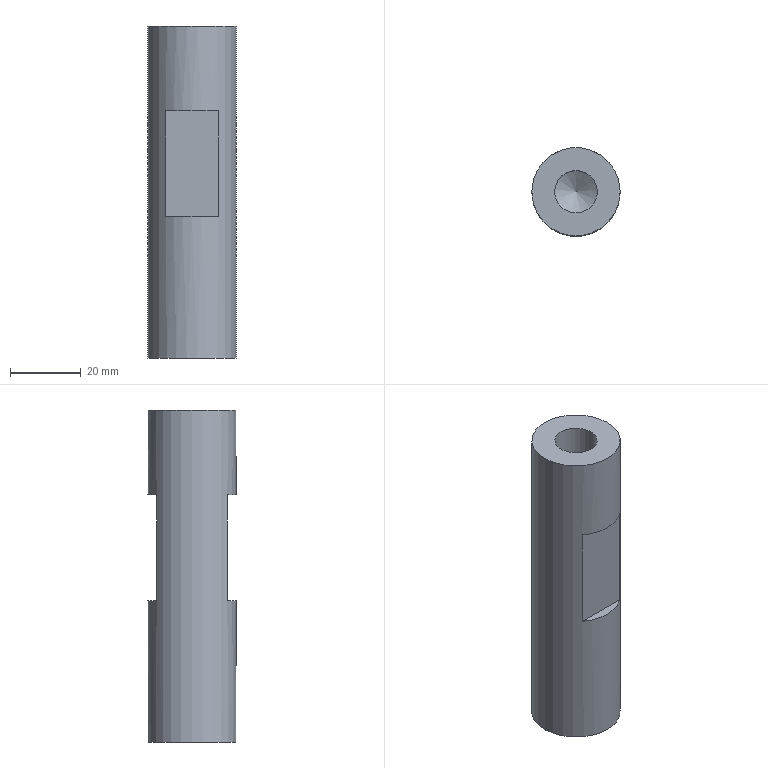Part | NX | features solid 2 | 1 solid | 13 faces | box 25 x 25 x 94 mm | volume 38683 mm3 | plane 8 | cylinder 3 | cone 2 | commonest cylinder face diameters 12 x2 25 x1
STEP:
#1=CARTESIAN_POINT('',(657.5,75.,-75.));
#2=VERTEX_POINT('',#1);
#3=CARTESIAN_POINT('',(670.,75.,-75.));
#4=DIRECTION('',(0.,0.,-1.));
#5=DIRECTION('',(-1.,0.,0.));
#6=AXIS2_PLACEMENT_3D('',#3,#4,#5);
#7=CIRCLE('',#6,12.5);
#8=EDGE_CURVE('',#2,#2,#7,.F.);
#9=ORIENTED_EDGE('',*,*,#8,.F.);
#10=EDGE_LOOP('',(#9));
#11=FACE_BOUND('',#10,.T.);
#12=CARTESIAN_POINT('',(682.5,75.,-169.));
#13=VERTEX_POINT('',#12);
#14=CARTESIAN_POINT('',(670.,75.,-169.));
#15=DIRECTION('',(0.,0.,1.));
#16=DIRECTION('',(1.,0.,0.));
#17=AXIS2_PLACEMENT_3D('',#14,#15,#16);
#18=CIRCLE('',#17,12.5);
#19=EDGE_CURVE('',#13,#13,#18,.T.);
#20=ORIENTED_EDGE('',*,*,#19,.T.);
#21=EDGE_LOOP('',(#20));
#22=FACE_BOUND('',#21,.T.);
#23=CARTESIAN_POINT('',(677.5,85.,-99.));
#24=VERTEX_POINT('',#23);
#25=CARTESIAN_POINT('',(677.5,85.,-129.));
#26=VERTEX_POINT('',#25);
#27=CARTESIAN_POINT('',(677.5,85.,-99.));
#28=DIRECTION('',(0.,0.,1.));
#29=VECTOR('',#28,1000.);
#30=LINE('',#27,#29);
#31=EDGE_CURVE('',#24,#26,#30,.F.);
#32=ORIENTED_EDGE('',*,*,#31,.F.);
#33=CARTESIAN_POINT('',(662.5,85.,-99.));
#34=VERTEX_POINT('',#33);
#35=CARTESIAN_POINT('',(670.,75.,-99.));
#36=DIRECTION('',(0.,0.,-1.));
#37=DIRECTION('',(-1.,0.,0.));
#38=AXIS2_PLACEMENT_3D('',#35,#36,#37);
#39=CIRCLE('',#38,12.5);
#40=EDGE_CURVE('',#34,#24,#39,.T.);
#41=ORIENTED_EDGE('',*,*,#40,.F.);
#42=CARTESIAN_POINT('',(662.5,85.,-129.));
#43=VERTEX_POINT('',#42);
#44=CARTESIAN_POINT('',(662.5,85.,-129.));
#45=DIRECTION('',(0.,0.,1.));
#46=VECTOR('',#45,1000.);
#47=LINE('',#44,#46);
#48=EDGE_CURVE('',#43,#34,#47,.T.);
#49=ORIENTED_EDGE('',*,*,#48,.F.);
#50=CARTESIAN_POINT('',(670.,75.,-129.));
#51=DIRECTION('',(0.,0.,-1.));
#52=DIRECTION('',(-1.,0.,0.));
#53=AXIS2_PLACEMENT_3D('',#50,#51,#52);
#54=CIRCLE('',#53,12.5);
#55=EDGE_CURVE('',#26,#43,#54,.F.);
#56=ORIENTED_EDGE('',*,*,#55,.F.);
#57=EDGE_LOOP('',(#32,#41,#49,#56));
#58=FACE_BOUND('',#57,.T.);
#59=CARTESIAN_POINT('',(662.5,65.,-99.));
#60=VERTEX_POINT('',#59);
#61=CARTESIAN_POINT('',(677.5,65.,-99.));
#62=VERTEX_POINT('',#61);
#63=CARTESIAN_POINT('',(670.,75.,-99.));
#64=DIRECTION('',(0.,0.,-1.));
#65=DIRECTION('',(-1.,0.,0.));
#66=AXIS2_PLACEMENT_3D('',#63,#64,#65);
#67=CIRCLE('',#66,12.5);
#68=EDGE_CURVE('',#60,#62,#67,.F.);
#69=ORIENTED_EDGE('',*,*,#68,.T.);
#70=CARTESIAN_POINT('',(677.5,65.,-129.));
#71=VERTEX_POINT('',#70);
#72=CARTESIAN_POINT('',(677.5,65.,-99.));
#73=DIRECTION('',(0.,0.,1.));
#74=VECTOR('',#73,1000.);
#75=LINE('',#72,#74);
#76=EDGE_CURVE('',#62,#71,#75,.F.);
#77=ORIENTED_EDGE('',*,*,#76,.T.);
#78=CARTESIAN_POINT('',(662.5,65.,-129.));
#79=VERTEX_POINT('',#78);
#80=CARTESIAN_POINT('',(670.,75.,-129.));
#81=DIRECTION('',(0.,0.,-1.));
#82=DIRECTION('',(-1.,0.,0.));
#83=AXIS2_PLACEMENT_3D('',#80,#81,#82);
#84=CIRCLE('',#83,12.5);
#85=EDGE_CURVE('',#71,#79,#84,.T.);
#86=ORIENTED_EDGE('',*,*,#85,.T.);
#87=CARTESIAN_POINT('',(662.5,65.,-129.));
#88=DIRECTION('',(0.,0.,1.));
#89=VECTOR('',#88,1000.);
#90=LINE('',#87,#89);
#91=EDGE_CURVE('',#79,#60,#90,.T.);
#92=ORIENTED_EDGE('',*,*,#91,.T.);
#93=EDGE_LOOP('',(#69,#77,#86,#92));
#94=FACE_BOUND('',#93,.T.);
#95=CARTESIAN_POINT('',(670.,75.,-169.));
#96=DIRECTION('',(0.,0.,1.));
#97=DIRECTION('',(0.,1.,0.));
#98=AXIS2_PLACEMENT_3D('',#95,#96,#97);
#99=CYLINDRICAL_SURFACE('',#98,12.5);
#100=ADVANCED_FACE('',(#11,#22,#58,#94),#99,.T.);
#101=CARTESIAN_POINT('',(670.,81.,-169.));
#102=VERTEX_POINT('',#101);
#103=CARTESIAN_POINT('',(670.,75.,-169.));
#104=DIRECTION('',(0.,0.,1.));
#105=DIRECTION('',(0.,1.,0.));
#106=AXIS2_PLACEMENT_3D('',#103,#104,#105);
#107=CIRCLE('',#106,6.);
#108=EDGE_CURVE('',#102,#102,#107,.T.);
#109=ORIENTED_EDGE('',*,*,#108,.T.);
#110=EDGE_LOOP('',(#109));
#111=FACE_BOUND('',#110,.T.);
#112=ORIENTED_EDGE('',*,*,#19,.F.);
#113=EDGE_LOOP('',(#112));
#114=FACE_BOUND('',#113,.T.);
#115=CARTESIAN_POINT('',(670.,75.,-169.));
#116=DIRECTION('',(0.,0.,1.));
#117=DIRECTION('',(0.,1.,0.));
#118=AXIS2_PLACEMENT_3D('',#115,#116,#117);
#119=PLANE('',#118);
#120=ADVANCED_FACE('',(#111,#114),#119,.F.);
#121=CARTESIAN_POINT('',(670.,69.,-75.));
#122=VERTEX_POINT('',#121);
#123=CARTESIAN_POINT('',(670.,75.,-75.));
#124=DIRECTION('',(0.,0.,-1.));
#125=DIRECTION('',(0.,-1.,0.));
#126=AXIS2_PLACEMENT_3D('',#123,#124,#125);
#127=CIRCLE('',#126,6.);
#128=EDGE_CURVE('',#122,#122,#127,.T.);
#129=ORIENTED_EDGE('',*,*,#128,.T.);
#130=EDGE_LOOP('',(#129));
#131=FACE_BOUND('',#130,.T.);
#132=ORIENTED_EDGE('',*,*,#8,.T.);
#133=EDGE_LOOP('',(#132));
#134=FACE_BOUND('',#133,.T.);
#135=CARTESIAN_POINT('',(520.,-10.,-75.));
#136=DIRECTION('',(0.,0.,-1.));
#137=DIRECTION('',(-1.,0.,0.));
#138=AXIS2_PLACEMENT_3D('',#135,#136,#137);
#139=PLANE('',#138);
#140=ADVANCED_FACE('',(#131,#134),#139,.F.);
#141=CARTESIAN_POINT('',(670.,69.,-95.));
#142=VERTEX_POINT('',#141);
#143=CARTESIAN_POINT('',(670.,75.,-95.));
#144=DIRECTION('',(0.,0.,-1.));
#145=DIRECTION('',(0.,-1.,0.));
#146=AXIS2_PLACEMENT_3D('',#143,#144,#145);
#147=CIRCLE('',#146,6.);
#148=EDGE_CURVE('',#142,#142,#147,.T.);
#149=ORIENTED_EDGE('',*,*,#148,.F.);
#150=EDGE_LOOP('',(#149));
#151=FACE_BOUND('',#150,.T.);
#152=CARTESIAN_POINT('',(670.,75.,-98.605));
#153=VERTEX_POINT('',#152);
#154=VERTEX_LOOP('',#153);
#155=FACE_BOUND('',#154,.T.);
#156=CARTESIAN_POINT('',(670.,75.,-95.));
#157=DIRECTION('',(0.,0.,1.));
#158=DIRECTION('',(0.,1.,0.));
#159=AXIS2_PLACEMENT_3D('',#156,#157,#158);
#160=CONICAL_SURFACE('',#159,6.,1.03);
#161=ADVANCED_FACE('',(#151,#155),#160,.F.);
#162=ORIENTED_EDGE('',*,*,#148,.T.);
#163=EDGE_LOOP('',(#162));
#164=FACE_BOUND('',#163,.T.);
#165=ORIENTED_EDGE('',*,*,#128,.F.);
#166=EDGE_LOOP('',(#165));
#167=FACE_BOUND('',#166,.T.);
#168=CARTESIAN_POINT('',(670.,75.,-65.));
#169=DIRECTION('',(0.,0.,-1.));
#170=DIRECTION('',(0.,-1.,0.));
#171=AXIS2_PLACEMENT_3D('',#168,#169,#170);
#172=CYLINDRICAL_SURFACE('',#171,6.);
#173=ADVANCED_FACE('',(#164,#167),#172,.F.);
#174=CARTESIAN_POINT('',(670.,81.,-139.));
#175=VERTEX_POINT('',#174);
#176=CARTESIAN_POINT('',(670.,75.,-139.));
#177=DIRECTION('',(0.,0.,1.));
#178=DIRECTION('',(0.,1.,0.));
#179=AXIS2_PLACEMENT_3D('',#176,#177,#178);
#180=CIRCLE('',#179,6.);
#181=EDGE_CURVE('',#175,#175,#180,.T.);
#182=ORIENTED_EDGE('',*,*,#181,.F.);
#183=EDGE_LOOP('',(#182));
#184=FACE_BOUND('',#183,.T.);
#185=CARTESIAN_POINT('',(670.,75.,-135.395));
#186=VERTEX_POINT('',#185);
#187=VERTEX_LOOP('',#186);
#188=FACE_BOUND('',#187,.T.);
#189=CARTESIAN_POINT('',(670.,75.,-139.));
#190=DIRECTION('',(0.,0.,-1.));
#191=DIRECTION('',(0.,-1.,0.));
#192=AXIS2_PLACEMENT_3D('',#189,#190,#191);
#193=CONICAL_SURFACE('',#192,6.,1.03);
#194=ADVANCED_FACE('',(#184,#188),#193,.F.);
#195=ORIENTED_EDGE('',*,*,#181,.T.);
#196=EDGE_LOOP('',(#195));
#197=FACE_BOUND('',#196,.T.);
#198=ORIENTED_EDGE('',*,*,#108,.F.);
#199=EDGE_LOOP('',(#198));
#200=FACE_BOUND('',#199,.T.);
#201=CARTESIAN_POINT('',(670.,75.,-169.));
#202=DIRECTION('',(0.,0.,1.));
#203=DIRECTION('',(0.,1.,0.));
#204=AXIS2_PLACEMENT_3D('',#201,#202,#203);
#205=CYLINDRICAL_SURFACE('',#204,6.);
#206=ADVANCED_FACE('',(#197,#200),#205,.F.);
#207=ORIENTED_EDGE('',*,*,#55,.T.);
#208=CARTESIAN_POINT('',(655.,85.,-129.));
#209=DIRECTION('',(1.,0.,0.));
#210=VECTOR('',#209,1000.);
#211=LINE('',#208,#210);
#212=EDGE_CURVE('',#43,#26,#211,.T.);
#213=ORIENTED_EDGE('',*,*,#212,.T.);
#214=EDGE_LOOP('',(#207,#213));
#215=FACE_BOUND('',#214,.T.);
#216=CARTESIAN_POINT('',(655.,75.,-129.));
#217=DIRECTION('',(0.,0.,-1.));
#218=DIRECTION('',(1.,0.,0.));
#219=AXIS2_PLACEMENT_3D('',#216,#217,#218);
#220=PLANE('',#219);
#221=ADVANCED_FACE('',(#215),#220,.F.);
#222=ORIENTED_EDGE('',*,*,#40,.T.);
#223=CARTESIAN_POINT('',(655.,85.,-99.));
#224=DIRECTION('',(-1.,0.,0.));
#225=VECTOR('',#224,1000.);
#226=LINE('',#223,#225);
#227=EDGE_CURVE('',#34,#24,#226,.F.);
#228=ORIENTED_EDGE('',*,*,#227,.F.);
#229=EDGE_LOOP('',(#222,#228));
#230=FACE_BOUND('',#229,.T.);
#231=CARTESIAN_POINT('',(655.,75.,-99.));
#232=DIRECTION('',(0.,0.,-1.));
#233=DIRECTION('',(1.,0.,0.));
#234=AXIS2_PLACEMENT_3D('',#231,#232,#233);
#235=PLANE('',#234);
#236=ADVANCED_FACE('',(#230),#235,.T.);
#237=ORIENTED_EDGE('',*,*,#31,.T.);
#238=ORIENTED_EDGE('',*,*,#212,.F.);
#239=ORIENTED_EDGE('',*,*,#48,.T.);
#240=ORIENTED_EDGE('',*,*,#227,.T.);
#241=EDGE_LOOP('',(#237,#238,#239,#240));
#242=FACE_BOUND('',#241,.T.);
#243=CARTESIAN_POINT('',(655.,85.,-129.));
#244=DIRECTION('',(0.,-1.,0.));
#245=DIRECTION('',(0.,0.,1.));
#246=AXIS2_PLACEMENT_3D('',#243,#244,#245);
#247=PLANE('',#246);
#248=ADVANCED_FACE('',(#242),#247,.F.);
#249=CARTESIAN_POINT('',(655.,65.,-129.));
#250=DIRECTION('',(-1.,0.,0.));
#251=VECTOR('',#250,1000.);
#252=LINE('',#249,#251);
#253=EDGE_CURVE('',#79,#71,#252,.F.);
#254=ORIENTED_EDGE('',*,*,#253,.F.);
#255=ORIENTED_EDGE('',*,*,#85,.F.);
#256=EDGE_LOOP('',(#254,#255));
#257=FACE_BOUND('',#256,.T.);
#258=CARTESIAN_POINT('',(655.,75.,-129.));
#259=DIRECTION('',(0.,0.,-1.));
#260=DIRECTION('',(1.,0.,0.));
#261=AXIS2_PLACEMENT_3D('',#258,#259,#260);
#262=PLANE('',#261);
#263=ADVANCED_FACE('',(#257),#262,.F.);
#264=CARTESIAN_POINT('',(655.,65.,-99.));
#265=DIRECTION('',(1.,0.,0.));
#266=VECTOR('',#265,1000.);
#267=LINE('',#264,#266);
#268=EDGE_CURVE('',#60,#62,#267,.T.);
#269=ORIENTED_EDGE('',*,*,#268,.T.);
#270=ORIENTED_EDGE('',*,*,#68,.F.);
#271=EDGE_LOOP('',(#269,#270));
#272=FACE_BOUND('',#271,.T.);
#273=CARTESIAN_POINT('',(655.,75.,-99.));
#274=DIRECTION('',(0.,0.,-1.));
#275=DIRECTION('',(1.,0.,0.));
#276=AXIS2_PLACEMENT_3D('',#273,#274,#275);
#277=PLANE('',#276);
#278=ADVANCED_FACE('',(#272),#277,.T.);
#279=ORIENTED_EDGE('',*,*,#268,.F.);
#280=ORIENTED_EDGE('',*,*,#91,.F.);
#281=ORIENTED_EDGE('',*,*,#253,.T.);
#282=ORIENTED_EDGE('',*,*,#76,.F.);
#283=EDGE_LOOP('',(#279,#280,#281,#282));
#284=FACE_BOUND('',#283,.T.);
#285=CARTESIAN_POINT('',(655.,65.,-129.));
#286=DIRECTION('',(0.,-1.,0.));
#287=DIRECTION('',(0.,0.,1.));
#288=AXIS2_PLACEMENT_3D('',#285,#286,#287);
#289=PLANE('',#288);
#290=ADVANCED_FACE('',(#284),#289,.T.);
#291=CLOSED_SHELL('',(#100,#120,#140,#161,#173,#194,#206,#221,#236,#248,#263,#278,#290));
#292=MANIFOLD_SOLID_BREP('',#291);
#293=(LENGTH_UNIT()NAMED_UNIT(*)SI_UNIT(.MILLI.,.METRE.));
#294=UNCERTAINTY_MEASURE_WITH_UNIT(LENGTH_MEASURE(0.00001),#293,'','');
#295=(NAMED_UNIT(*)PLANE_ANGLE_UNIT()SI_UNIT($,.RADIAN.));
#296=(NAMED_UNIT(*)SI_UNIT($,.STERADIAN.)SOLID_ANGLE_UNIT());
#297=(GEOMETRIC_REPRESENTATION_CONTEXT(3)GLOBAL_UNCERTAINTY_ASSIGNED_CONTEXT((#294))GLOBAL_UNIT_ASSIGNED_CONTEXT((#293,#295,#296))REPRESENTATION_CONTEXT('',''));
#298=ADVANCED_BREP_SHAPE_REPRESENTATION('',(#292),#297);